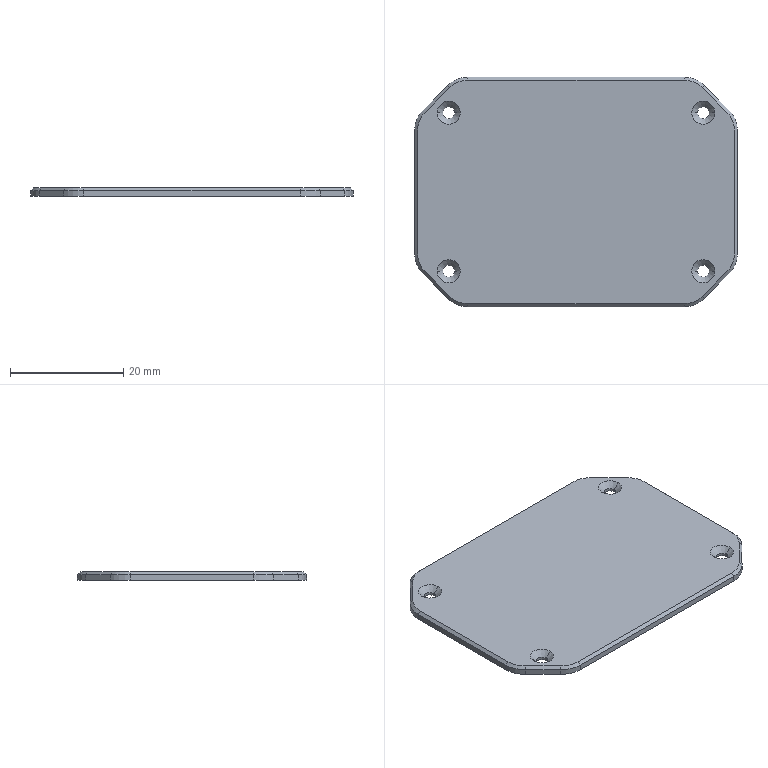NC program | NX | posted with a generic post | part box 57 x 40.5 x 1.5 mm
Lines 1492 to 2967 of 7802:
(PLANAR_PROFILE_COPY_4 , TOOL : D4)
N2916 T01 M6
N2918 G54
N2920 G17 G0 G90 X-245.9 Y31.609 S6500 M3
N2922 G43 Z20. H1
N2924 Z0.1
N2926 G94 G1 Y8.668 Z0.06 F1200.
N2928 X-246.173 Y7.266 Z0.057
N2930 X-246.719 Y5.947 Z0.055
N2932 X-247.518 Y4.763 Z0.052
N2934 X-252.763 Y-0.482 Z0.04
N2936 X-253.947 Y-1.281 Z0.037
N2938 X-255.266 Y-1.827 Z0.035
N2940 X-256.668 Y-2.1 Z0.032
N2942 X-296.332 Z-0.037
N2944 X-297.734 Y-1.827 Z-0.04
N2946 X-299.053 Y-1.281 Z-0.042
N2948 X-300.237 Y-0.482 Z-0.045
N2950 X-305.482 Y4.763 Z-0.058
N2952 X-306.281 Y5.947 Z-0.06
N2954 X-306.827 Y7.266 Z-0.063
N2956 X-307.1 Y8.668 Z-0.065
N2958 Y31.832 Z-0.106
N2960 X-306.827 Y33.234 Z-0.108
N2962 X-306.281 Y34.553 Z-0.11
N2964 X-305.482 Y35.737 Z-0.113
N2966 X-300.237 Y40.982 Z-0.126
N2968 X-299.053 Y41.781 Z-0.128
N2970 X-297.734 Y42.327 Z-0.131
N2972 X-296.332 Y42.6 Z-0.133
N2974 X-256.668 Z-0.203
N2976 X-255.266 Y42.327 Z-0.205
N2978 X-253.947 Y41.781 Z-0.208
N2980 X-252.763 Y40.982 Z-0.21
N2982 X-247.518 Y35.737 Z-0.223
N2984 X-246.719 Y34.553 Z-0.226
N2986 X-246.173 Y33.234 Z-0.228
N2988 X-245.9 Y31.832 Z-0.231
N2990 Y8.668 Z-0.271
N2992 X-246.173 Y7.266 Z-0.273
N2994 X-246.719 Y5.947 Z-0.276
N2996 X-247.518 Y4.763 Z-0.278
N2998 X-252.763 Y-0.482 Z-0.291
N3000 X-253.947 Y-1.281 Z-0.294
N3002 X-255.266 Y-1.827 Z-0.296
N3004 X-256.668 Y-2.1 Z-0.299
N3006 X-257.321 Z-0.3
N3008 X-295.679 F2000.
N3010 G2 X-300.699 Y-0.02 R7.1
N3012 G1 X-305.02 Y4.301
N3014 G2 X-307.1 Y9.321 R7.1
N3016 G1 Y31.179
N3018 G2 X-305.02 Y36.199 R7.1
N3020 G1 X-300.699 Y40.52
N3022 G2 X-295.679 Y42.6 R7.1
N3024 G1 X-257.321
N3026 G2 X-252.301 Y40.52 R7.1
N3028 G1 X-247.98 Y36.199
N3030 G2 X-245.9 Y31.179 R7.1
N3032 G1 Y9.321
N3034 G2 X-247.98 Y4.301 R7.1
N3036 G1 X-252.301 Y-0.02
N3038 G2 X-257.321 Y-2.1 R7.1
N3040 G1 Z-0.2
N3042 G0 Z20.
N3044 X-245.9 Y31.609
N3046 Z-0.2
N3048 G1 Y8.668 Z-0.24 F1200.
N3050 X-246.173 Y7.266 Z-0.243
N3052 X-246.719 Y5.947 Z-0.245
N3054 X-247.518 Y4.763 Z-0.248
N3056 X-252.763 Y-0.482 Z-0.26
N3058 X-253.947 Y-1.281 Z-0.263
N3060 X-255.266 Y-1.827 Z-0.265
N3062 X-256.668 Y-2.1 Z-0.268
N3064 X-296.332 Z-0.337
N3066 X-297.734 Y-1.827 Z-0.34
N3068 X-299.053 Y-1.281 Z-0.342
N3070 X-300.237 Y-0.482 Z-0.345
N3072 X-305.482 Y4.763 Z-0.358
N3074 X-306.281 Y5.947 Z-0.36
N3076 X-306.827 Y7.266 Z-0.363
N3078 X-307.1 Y8.668 Z-0.365
N3080 Y31.832 Z-0.406
N3082 X-306.827 Y33.234 Z-0.408
N3084 X-306.281 Y34.553 Z-0.41
N3086 X-305.482 Y35.737 Z-0.413
N3088 X-300.237 Y40.982 Z-0.426
N3090 X-299.053 Y41.781 Z-0.428
N3092 X-297.734 Y42.327 Z-0.431
N3094 X-296.332 Y42.6 Z-0.433
N3096 X-256.668 Z-0.503
N3098 X-255.266 Y42.327 Z-0.505
N3100 X-253.947 Y41.781 Z-0.508
N3102 X-252.763 Y40.982 Z-0.51
N3104 X-247.518 Y35.737 Z-0.523
N3106 X-246.719 Y34.553 Z-0.526
N3108 X-246.173 Y33.234 Z-0.528
N3110 X-245.9 Y31.832 Z-0.531
N3112 Y8.668 Z-0.571
N3114 X-246.173 Y7.266 Z-0.573
N3116 X-246.719 Y5.947 Z-0.576
N3118 X-247.518 Y4.763 Z-0.578
N3120 X-252.763 Y-0.482 Z-0.591
N3122 X-253.947 Y-1.281 Z-0.594
N3124 X-255.266 Y-1.827 Z-0.596
N3126 X-256.668 Y-2.1 Z-0.599
N3128 X-257.321 Z-0.6
N3130 X-295.679 F2000.
N3132 G2 X-300.699 Y-0.02 R7.1
N3134 G1 X-305.02 Y4.301
N3136 G2 X-307.1 Y9.321 R7.1
N3138 G1 Y31.179
N3140 G2 X-305.02 Y36.199 R7.1
N3142 G1 X-300.699 Y40.52
N3144 G2 X-295.679 Y42.6 R7.1
N3146 G1 X-257.321
N3148 G2 X-252.301 Y40.52 R7.1
N3150 G1 X-247.98 Y36.199
N3152 G2 X-245.9 Y31.179 R7.1
N3154 G1 Y9.321
N3156 G2 X-247.98 Y4.301 R7.1
N3158 G1 X-252.301 Y-0.02
N3160 G2 X-257.321 Y-2.1 R7.1
N3162 G1 Z-0.5
N3164 G0 Z20.
N3166 X-245.9 Y31.609
N3168 Z-0.5
N3170 G1 Y8.668 Z-0.54 F1200.
N3172 X-246.173 Y7.266 Z-0.543
N3174 X-246.719 Y5.947 Z-0.545
N3176 X-247.518 Y4.763 Z-0.548
N3178 X-252.763 Y-0.482 Z-0.56
N3180 X-253.947 Y-1.281 Z-0.563
N3182 X-255.266 Y-1.827 Z-0.565
N3184 X-256.668 Y-2.1 Z-0.568
N3186 X-296.332 Z-0.637
N3188 X-297.734 Y-1.827 Z-0.64
N3190 X-299.053 Y-1.281 Z-0.642
N3192 X-300.237 Y-0.482 Z-0.645
N3194 X-305.482 Y4.763 Z-0.658
N3196 X-306.281 Y5.947 Z-0.66
N3198 X-306.827 Y7.266 Z-0.663
N3200 X-307.1 Y8.668 Z-0.665
N3202 Y31.832 Z-0.706
N3204 X-306.827 Y33.234 Z-0.708
N3206 X-306.281 Y34.553 Z-0.71
N3208 X-305.482 Y35.737 Z-0.713
N3210 X-300.237 Y40.982 Z-0.726
N3212 X-299.053 Y41.781 Z-0.728
N3214 X-297.734 Y42.327 Z-0.731
N3216 X-296.332 Y42.6 Z-0.733
N3218 X-256.668 Z-0.803
N3220 X-255.266 Y42.327 Z-0.805
N3222 X-253.947 Y41.781 Z-0.808
N3224 X-252.763 Y40.982 Z-0.81
N3226 X-247.518 Y35.737 Z-0.823
N3228 X-246.719 Y34.553 Z-0.826
N3230 X-246.173 Y33.234 Z-0.828
N3232 X-245.9 Y31.832 Z-0.831
N3234 Y8.668 Z-0.871
N3236 X-246.173 Y7.266 Z-0.873
N3238 X-246.719 Y5.947 Z-0.876
N3240 X-247.518 Y4.763 Z-0.878
N3242 X-252.763 Y-0.482 Z-0.891
N3244 X-253.947 Y-1.281 Z-0.894
N3246 X-255.266 Y-1.827 Z-0.896
N3248 X-256.668 Y-2.1 Z-0.899
N3250 X-257.321 Z-0.9
N3252 X-295.679 F2000.
N3254 G2 X-300.699 Y-0.02 R7.1
N3256 G1 X-305.02 Y4.301
N3258 G2 X-307.1 Y9.321 R7.1
N3260 G1 Y31.179
N3262 G2 X-305.02 Y36.199 R7.1
N3264 G1 X-300.699 Y40.52
N3266 G2 X-295.679 Y42.6 R7.1
N3268 G1 X-257.321
N3270 G2 X-252.301 Y40.52 R7.1
N3272 G1 X-247.98 Y36.199
N3274 G2 X-245.9 Y31.179 R7.1
N3276 G1 Y9.321
N3278 G2 X-247.98 Y4.301 R7.1
N3280 G1 X-252.301 Y-0.02
N3282 G2 X-257.321 Y-2.1 R7.1
N3284 G1 Z-0.8
N3286 G0 Z20.
N3288 X-245.9 Y31.609
N3290 Z-0.8
N3292 G1 Y8.668 Z-0.84 F1200.
N3294 X-246.173 Y7.266 Z-0.843
N3296 X-246.719 Y5.947 Z-0.845
N3298 X-247.518 Y4.763 Z-0.848
N3300 X-252.763 Y-0.482 Z-0.86
N3302 X-253.947 Y-1.281 Z-0.863
N3304 X-255.266 Y-1.827 Z-0.865
N3306 X-256.668 Y-2.1 Z-0.868
N3308 X-296.332 Z-0.937
N3310 X-297.734 Y-1.827 Z-0.94
N3312 X-299.053 Y-1.281 Z-0.942
N3314 X-300.237 Y-0.482 Z-0.945
N3316 X-305.482 Y4.763 Z-0.958
N3318 X-306.281 Y5.947 Z-0.96
N3320 X-306.827 Y7.266 Z-0.963
N3322 X-307.1 Y8.668 Z-0.965
N3324 Y31.832 Z-1.006
N3326 X-306.827 Y33.234 Z-1.008
N3328 X-306.281 Y34.553 Z-1.01
N3330 X-305.482 Y35.737 Z-1.013
N3332 X-300.237 Y40.982 Z-1.026
N3334 X-299.053 Y41.781 Z-1.028
N3336 X-297.734 Y42.327 Z-1.031
N3338 X-296.332 Y42.6 Z-1.033
N3340 X-256.668 Z-1.103
N3342 X-255.266 Y42.327 Z-1.105
N3344 X-253.947 Y41.781 Z-1.108
N3346 X-252.763 Y40.982 Z-1.11
N3348 X-247.518 Y35.737 Z-1.123
N3350 X-246.719 Y34.553 Z-1.126
N3352 X-246.173 Y33.234 Z-1.128
N3354 X-245.9 Y31.832 Z-1.131
N3356 Y8.668 Z-1.171
N3358 X-246.173 Y7.266 Z-1.173
N3360 X-246.719 Y5.947 Z-1.176
N3362 X-247.518 Y4.763 Z-1.178
N3364 X-252.763 Y-0.482 Z-1.191
N3366 X-253.947 Y-1.281 Z-1.194
N3368 X-255.266 Y-1.827 Z-1.196
N3370 X-256.668 Y-2.1 Z-1.199
N3372 X-257.321 Z-1.2
N3374 X-295.679 F2000.
N3376 G2 X-300.699 Y-0.02 R7.1
N3378 G1 X-305.02 Y4.301
N3380 G2 X-307.1 Y9.321 R7.1
N3382 G1 Y31.179
N3384 G2 X-305.02 Y36.199 R7.1
N3386 G1 X-300.699 Y40.52
N3388 G2 X-295.679 Y42.6 R7.1
N3390 G1 X-257.321
N3392 G2 X-252.301 Y40.52 R7.1
N3394 G1 X-247.98 Y36.199
N3396 G2 X-245.9 Y31.179 R7.1
N3398 G1 Y9.321
N3400 G2 X-247.98 Y4.301 R7.1
N3402 G1 X-252.301 Y-0.02
N3404 G2 X-257.321 Y-2.1 R7.1
N3406 G1 Z-1.1
N3408 G0 Z20.
N3410 X-302.406 Y1.686
N3412 Z-1.1
N3414 G1 X-305.482 Y4.763 Z-1.108 F1200.
N3416 X-306.281 Y5.947 Z-1.11
N3418 X-306.827 Y7.266 Z-1.113
N3420 X-307.1 Y8.668 Z-1.115
N3422 Y31.832 Z-1.156
N3424 X-306.827 Y33.234 Z-1.158
N3426 X-306.281 Y34.553 Z-1.16
N3428 X-305.482 Y35.737 Z-1.163
N3430 X-300.237 Y40.982 Z-1.176
N3432 X-299.053 Y41.781 Z-1.178
N3434 X-297.734 Y42.327 Z-1.181
N3436 X-296.332 Y42.6 Z-1.183
N3438 X-256.668 Z-1.253
N3440 X-255.266 Y42.327 Z-1.255
N3442 X-253.947 Y41.781 Z-1.258
N3444 X-252.763 Y40.982 Z-1.26
N3446 X-247.518 Y35.737 Z-1.273
N3448 X-246.719 Y34.553 Z-1.276
N3450 X-246.173 Y33.234 Z-1.278
N3452 X-245.9 Y31.832 Z-1.281
N3454 Y8.668 Z-1.321
N3456 X-246.173 Y7.266 Z-1.323
N3458 X-246.719 Y5.947 Z-1.326
N3460 X-247.518 Y4.763 Z-1.328
N3462 X-252.763 Y-0.482 Z-1.341
N3464 X-253.947 Y-1.281 Z-1.344
N3466 X-255.266 Y-1.827 Z-1.346
N3468 X-256.668 Y-2.1 Z-1.349
N3470 X-257.321 Z-1.35
N3472 X-295.679 F2000.
N3474 G2 X-300.699 Y-0.02 R7.1
N3476 G1 X-305.02 Y4.301
N3478 G2 X-307.1 Y9.321 R7.1
N3480 G1 Y31.179
N3482 G2 X-305.02 Y36.199 R7.1
N3484 G1 X-300.699 Y40.52
N3486 G2 X-295.679 Y42.6 R7.1
N3488 G1 X-257.321
N3490 G2 X-252.301 Y40.52 R7.1
N3492 G1 X-247.98 Y36.199
N3494 G2 X-245.9 Y31.179 R7.1
N3496 G1 Y9.321
N3498 G2 X-247.98 Y4.301 R7.1
N3500 G1 X-252.301 Y-0.02
N3502 G2 X-257.321 Y-2.1 R7.1
N3504 G1 Z-1.25
N3506 G0 Z20.
(PLANAR_PROFILE_COPY_COPY_4 , TOOL : D4)
N3508 X-257.221
N3510 Z1.65
N3512 G1 Z-1.35 F800.
N3514 X-257.232 Y-2.049
N3516 X-257.27 Y-2.011
N3518 X-257.321 Y-2.
N3520 X-295.679
N3522 G2 X-300.629 Y0.05 R7.
N3524 G1 X-304.95 Y4.371
N3526 G2 X-307. Y9.321 R7.
N3528 G1 Y31.179
N3530 G2 X-304.95 Y36.129 R7.
N3532 G1 X-300.629 Y40.45
N3534 G2 X-295.679 Y42.5 R7.
N3536 G1 X-257.321
N3538 G2 X-252.371 Y40.45 R7.
N3540 G1 X-248.05 Y36.129
N3542 G2 X-246. Y31.179 R7.
N3544 G1 Y9.321
N3546 G2 X-248.05 Y4.371 R7.
N3548 G1 X-252.371 Y0.05
N3550 G2 X-257.321 Y-2. R7.
N3552 G1 X-257.373 Y-2.011
N3554 X-257.41 Y-2.049
N3556 X-257.421 Y-2.1
N3558 Z1.65
N3560 G0 Z20.
N3562 M5
(PLANAR_PROFILE_COPY_COPY_COPY_3 , TOOL : D3倒角)
N3564 T02 M6
N3566 G54
N3568 G17 G0 G90 X-255.321 Y-2.6 S4500 M3
N3570 G43 Z20. H2
N3572 Z2.
N3574 G94 G1 Z-1. F800.
N3576 G3 X-257.321 Y-0.6 R2.
N3578 G1 X-295.679
N3580 G2 X-299.639 Y1.04 R5.6
N3582 G1 X-303.96 Y5.361
N3584 G2 X-305.6 Y9.321 R5.6
N3586 G1 Y31.179
N3588 G2 X-303.96 Y35.139 R5.6
N3590 G1 X-299.639 Y39.46
N3592 G2 X-295.679 Y41.1 R5.6
N3594 G1 X-257.321
N3596 G2 X-253.361 Y39.46 R5.6
N3598 G1 X-249.04 Y35.139
N3600 G2 X-247.4 Y31.179 R5.6
N3602 G1 Y9.321
N3604 G2 X-249.04 Y5.361 R5.6
N3606 G1 X-253.361 Y1.04
N3608 G2 X-257.321 Y-0.6 R5.6
N3610 G3 X-259.321 Y-2.6 R2.
N3612 G1 Z2.
N3614 G0 Z20.
N3616 M5
(PLANAR_PROFILE_COPY_5 , TOOL : D4)
N3618 T01 M6
N3620 G54
N3622 G17 G0 G90 X2.1 Y91.609 S6500 M3
N3624 G43 Z20. H1
N3626 Z0.1
N3628 G94 G1 Y68.668 Z0.06 F1200.
N3630 X1.827 Y67.266 Z0.057
N3632 X1.281 Y65.947 Z0.055
N3634 X0.482 Y64.763 Z0.052
N3636 X-4.763 Y59.518 Z0.04
N3638 X-5.947 Y58.719 Z0.037
N3640 X-7.266 Y58.173 Z0.035
N3642 X-8.668 Y57.9 Z0.032
N3644 X-48.332 Z-0.037
N3646 X-49.734 Y58.173 Z-0.04
N3648 X-51.053 Y58.719 Z-0.042
N3650 X-52.237 Y59.518 Z-0.045
N3652 X-57.482 Y64.763 Z-0.058
N3654 X-58.281 Y65.947 Z-0.06
N3656 X-58.827 Y67.266 Z-0.063
N3658 X-59.1 Y68.668 Z-0.065
N3660 Y91.832 Z-0.106
N3662 X-58.827 Y93.234 Z-0.108
N3664 X-58.281 Y94.553 Z-0.11
N3666 X-57.482 Y95.737 Z-0.113
N3668 X-52.237 Y100.982 Z-0.126
N3670 X-51.053 Y101.781 Z-0.128
N3672 X-49.734 Y102.327 Z-0.131
N3674 X-48.332 Y102.6 Z-0.133
N3676 X-8.668 Z-0.203
N3678 X-7.266 Y102.327 Z-0.205
N3680 X-5.947 Y101.781 Z-0.208
N3682 X-4.763 Y100.982 Z-0.21
N3684 X0.482 Y95.737 Z-0.223
N3686 X1.281 Y94.553 Z-0.226
N3688 X1.827 Y93.234 Z-0.228
N3690 X2.1 Y91.832 Z-0.231
N3692 Y68.668 Z-0.271
N3694 X1.827 Y67.266 Z-0.273
N3696 X1.281 Y65.947 Z-0.276
N3698 X0.482 Y64.763 Z-0.278
N3700 X-4.763 Y59.518 Z-0.291
N3702 X-5.947 Y58.719 Z-0.294
N3704 X-7.266 Y58.173 Z-0.296
N3706 X-8.668 Y57.9 Z-0.299
N3708 X-9.321 Z-0.3
N3710 X-47.679 F2000.
N3712 G2 X-52.699 Y59.98 R7.1
N3714 G1 X-57.02 Y64.301
N3716 G2 X-59.1 Y69.321 R7.1
N3718 G1 Y91.179
N3720 G2 X-57.02 Y96.199 R7.1
N3722 G1 X-52.699 Y100.52
N3724 G2 X-47.679 Y102.6 R7.1
N3726 G1 X-9.321
N3728 G2 X-4.301 Y100.52 R7.1
N3730 G1 X0.02 Y96.199
N3732 G2 X2.1 Y91.179 R7.1
N3734 G1 Y69.321
N3736 G2 X0.02 Y64.301 R7.1
N3738 G1 X-4.301 Y59.98
N3740 G2 X-9.321 Y57.9 R7.1
N3742 G1 Z-0.2
N3744 G0 Z20.
N3746 X2.1 Y91.609
N3748 Z-0.2
N3750 G1 Y68.668 Z-0.24 F1200.
N3752 X1.827 Y67.266 Z-0.243
N3754 X1.281 Y65.947 Z-0.245
N3756 X0.482 Y64.763 Z-0.248
N3758 X-4.763 Y59.518 Z-0.26
N3760 X-5.947 Y58.719 Z-0.263
N3762 X-7.266 Y58.173 Z-0.265
N3764 X-8.668 Y57.9 Z-0.268
N3766 X-48.332 Z-0.337
N3768 X-49.734 Y58.173 Z-0.34
N3770 X-51.053 Y58.719 Z-0.342
N3772 X-52.237 Y59.518 Z-0.345
N3774 X-57.482 Y64.763 Z-0.358
N3776 X-58.281 Y65.947 Z-0.36
N3778 X-58.827 Y67.266 Z-0.363
N3780 X-59.1 Y68.668 Z-0.365
N3782 Y91.832 Z-0.406
N3784 X-58.827 Y93.234 Z-0.408
N3786 X-58.281 Y94.553 Z-0.41
N3788 X-57.482 Y95.737 Z-0.413
N3790 X-52.237 Y100.982 Z-0.426
N3792 X-51.053 Y101.781 Z-0.428
N3794 X-49.734 Y102.327 Z-0.431
N3796 X-48.332 Y102.6 Z-0.433
N3798 X-8.668 Z-0.503
N3800 X-7.266 Y102.327 Z-0.505
N3802 X-5.947 Y101.781 Z-0.508
N3804 X-4.763 Y100.982 Z-0.51
N3806 X0.482 Y95.737 Z-0.523
N3808 X1.281 Y94.553 Z-0.526
N3810 X1.827 Y93.234 Z-0.528
N3812 X2.1 Y91.832 Z-0.531
N3814 Y68.668 Z-0.571
N3816 X1.827 Y67.266 Z-0.573
N3818 X1.281 Y65.947 Z-0.576
N3820 X0.482 Y64.763 Z-0.578
N3822 X-4.763 Y59.518 Z-0.591
N3824 X-5.947 Y58.719 Z-0.594
N3826 X-7.266 Y58.173 Z-0.596
N3828 X-8.668 Y57.9 Z-0.599
N3830 X-9.321 Z-0.6
N3832 X-47.679 F2000.
N3834 G2 X-52.699 Y59.98 R7.1
N3836 G1 X-57.02 Y64.301
N3838 G2 X-59.1 Y69.321 R7.1
N3840 G1 Y91.179
N3842 G2 X-57.02 Y96.199 R7.1
N3844 G1 X-52.699 Y100.52
N3846 G2 X-47.679 Y102.6 R7.1
N3848 G1 X-9.321
N3850 G2 X-4.301 Y100.52 R7.1
N3852 G1 X0.02 Y96.199
N3854 G2 X2.1 Y91.179 R7.1
N3856 G1 Y69.321
N3858 G2 X0.02 Y64.301 R7.1
N3860 G1 X-4.301 Y59.98
N3862 G2 X-9.321 Y57.9 R7.1
N3864 G1 Z-0.5
N3866 G0 Z20.
N3868 X2.1 Y91.609
N3870 Z-0.5
N3872 G1 Y68.668 Z-0.54 F1200.
N3874 X1.827 Y67.266 Z-0.543
N3876 X1.281 Y65.947 Z-0.545
N3878 X0.482 Y64.763 Z-0.548
N3880 X-4.763 Y59.518 Z-0.56
N3882 X-5.947 Y58.719 Z-0.563
N3884 X-7.266 Y58.173 Z-0.565
N3886 X-8.668 Y57.9 Z-0.568
N3888 X-48.332 Z-0.637
N3890 X-49.734 Y58.173 Z-0.64
N3892 X-51.053 Y58.719 Z-0.642
N3894 X-52.237 Y59.518 Z-0.645
N3896 X-57.482 Y64.763 Z-0.658
N3898 X-58.281 Y65.947 Z-0.66
N3900 X-58.827 Y67.266 Z-0.663
N3902 X-59.1 Y68.668 Z-0.665
N3904 Y91.832 Z-0.706
N3906 X-58.827 Y93.234 Z-0.708
N3908 X-58.281 Y94.553 Z-0.71
N3910 X-57.482 Y95.737 Z-0.713
N3912 X-52.237 Y100.982 Z-0.726
N3914 X-51.053 Y101.781 Z-0.728
N3916 X-49.734 Y102.327 Z-0.731
N3918 X-48.332 Y102.6 Z-0.733
N3920 X-8.668 Z-0.803
N3922 X-7.266 Y102.327 Z-0.805
N3924 X-5.947 Y101.781 Z-0.808
N3926 X-4.763 Y100.982 Z-0.81
N3928 X0.482 Y95.737 Z-0.823
N3930 X1.281 Y94.553 Z-0.826
N3932 X1.827 Y93.234 Z-0.828
N3934 X2.1 Y91.832 Z-0.831
N3936 Y68.668 Z-0.871
N3938 X1.827 Y67.266 Z-0.873
N3940 X1.281 Y65.947 Z-0.876
N3942 X0.482 Y64.763 Z-0.878
N3944 X-4.763 Y59.518 Z-0.891
N3946 X-5.947 Y58.719 Z-0.894
N3948 X-7.266 Y58.173 Z-0.896
N3950 X-8.668 Y57.9 Z-0.899
N3952 X-9.321 Z-0.9
N3954 X-47.679 F2000.
N3956 G2 X-52.699 Y59.98 R7.1
N3958 G1 X-57.02 Y64.301
N3960 G2 X-59.1 Y69.321 R7.1
N3962 G1 Y91.179
N3964 G2 X-57.02 Y96.199 R7.1
N3966 G1 X-52.699 Y100.52
N3968 G2 X-47.679 Y102.6 R7.1
N3970 G1 X-9.321
N3972 G2 X-4.301 Y100.52 R7.1
N3974 G1 X0.02 Y96.199
N3976 G2 X2.1 Y91.179 R7.1
N3978 G1 Y69.321
N3980 G2 X0.02 Y64.301 R7.1
N3982 G1 X-4.301 Y59.98
N3984 G2 X-9.321 Y57.9 R7.1
N3986 G1 Z-0.8
N3988 G0 Z20.
N3990 X2.1 Y91.609
N3992 Z-0.8
N3994 G1 Y68.668 Z-0.84 F1200.
N3996 X1.827 Y67.266 Z-0.843
N3998 X1.281 Y65.947 Z-0.845
N4000 X0.482 Y64.763 Z-0.848
N4002 X-4.763 Y59.518 Z-0.86
N4004 X-5.947 Y58.719 Z-0.863
N4006 X-7.266 Y58.173 Z-0.865
N4008 X-8.668 Y57.9 Z-0.868
N4010 X-48.332 Z-0.937
N4012 X-49.734 Y58.173 Z-0.94
N4014 X-51.053 Y58.719 Z-0.942
N4016 X-52.237 Y59.518 Z-0.945
N4018 X-57.482 Y64.763 Z-0.958
N4020 X-58.281 Y65.947 Z-0.96
N4022 X-58.827 Y67.266 Z-0.963
N4024 X-59.1 Y68.668 Z-0.965
N4026 Y91.832 Z-1.006
N4028 X-58.827 Y93.234 Z-1.008
N4030 X-58.281 Y94.553 Z-1.01
N4032 X-57.482 Y95.737 Z-1.013
N4034 X-52.237 Y100.982 Z-1.026
N4036 X-51.053 Y101.781 Z-1.028
N4038 X-49.734 Y102.327 Z-1.031
N4040 X-48.332 Y102.6 Z-1.033
N4042 X-8.668 Z-1.103
N4044 X-7.266 Y102.327 Z-1.105
N4046 X-5.947 Y101.781 Z-1.108
N4048 X-4.763 Y100.982 Z-1.11
N4050 X0.482 Y95.737 Z-1.123
N4052 X1.281 Y94.553 Z-1.126
N4054 X1.827 Y93.234 Z-1.128
N4056 X2.1 Y91.832 Z-1.131
N4058 Y68.668 Z-1.171
N4060 X1.827 Y67.266 Z-1.173
N4062 X1.281 Y65.947 Z-1.176
N4064 X0.482 Y64.763 Z-1.178
N4066 X-4.763 Y59.518 Z-1.191
N4068 X-5.947 Y58.719 Z-1.194
N4070 X-7.266 Y58.173 Z-1.196
N4072 X-8.668 Y57.9 Z-1.199
N4074 X-9.321 Z-1.2
N4076 X-47.679 F2000.
N4078 G2 X-52.699 Y59.98 R7.1
N4080 G1 X-57.02 Y64.301
N4082 G2 X-59.1 Y69.321 R7.1
N4084 G1 Y91.179
N4086 G2 X-57.02 Y96.199 R7.1
N4088 G1 X-52.699 Y100.52
N4090 G2 X-47.679 Y102.6 R7.1
N4092 G1 X-9.321
N4094 G2 X-4.301 Y100.52 R7.1
N4096 G1 X0.02 Y96.199
N4098 G2 X2.1 Y91.179 R7.1
N4100 G1 Y69.321
N4102 G2 X0.02 Y64.301 R7.1
N4104 G1 X-4.301 Y59.98
N4106 G2 X-9.321 Y57.9 R7.1
N4108 G1 Z-1.1
N4110 G0 Z20.
N4112 X2.1 Y91.609
N4114 Z-1.1
N4116 G1 Y68.668 Z-1.14 F1200.
N4118 X1.827 Y67.266 Z-1.143
N4120 X1.281 Y65.947 Z-1.145
N4122 X0.482 Y64.763 Z-1.148
N4124 X-4.763 Y59.518 Z-1.16
N4126 X-5.947 Y58.719 Z-1.163
N4128 X-7.266 Y58.173 Z-1.165
N4130 X-8.668 Y57.9 Z-1.168
N4132 X-48.332 Z-1.237
N4134 X-49.734 Y58.173 Z-1.24
N4136 X-51.053 Y58.719 Z-1.242
N4138 X-52.237 Y59.518 Z-1.245
N4140 X-57.482 Y64.763 Z-1.258
N4142 X-58.281 Y65.947 Z-1.26
N4144 X-58.827 Y67.266 Z-1.263
N4146 X-59.1 Y68.668 Z-1.265
N4148 Y91.832 Z-1.306
N4150 X-58.827 Y93.234 Z-1.308
N4152 X-58.281 Y94.553 Z-1.31
N4154 X-57.482 Y95.737 Z-1.313
N4156 X-52.237 Y100.982 Z-1.326
N4158 X-51.053 Y101.781 Z-1.328
N4160 X-49.734 Y102.327 Z-1.331
N4162 X-48.332 Y102.6 Z-1.333
N4164 X-8.668 Z-1.403
N4166 X-7.266 Y102.327 Z-1.405
N4168 X-5.947 Y101.781 Z-1.408
N4170 X-4.763 Y100.982 Z-1.41
N4172 X0.482 Y95.737 Z-1.423
N4174 X1.281 Y94.553 Z-1.426
N4176 X1.827 Y93.234 Z-1.428
N4178 X2.1 Y91.832 Z-1.431
N4180 Y68.668 Z-1.471
N4182 X1.827 Y67.266 Z-1.473
N4184 X1.281 Y65.947 Z-1.476
N4186 X0.482 Y64.763 Z-1.478
N4188 X-4.763 Y59.518 Z-1.491
N4190 X-5.947 Y58.719 Z-1.494
N4192 X-7.266 Y58.173 Z-1.496
N4194 X-8.668 Y57.9 Z-1.499
N4196 X-9.321 Z-1.5
N4198 X-47.679 F2000.
N4200 G2 X-52.699 Y59.98 R7.1
N4202 G1 X-57.02 Y64.301
N4204 G2 X-59.1 Y69.321 R7.1
N4206 G1 Y91.179
N4208 G2 X-57.02 Y96.199 R7.1
N4210 G1 X-52.699 Y100.52
N4212 G2 X-47.679 Y102.6 R7.1
N4214 G1 X-9.321
N4216 G2 X-4.301 Y100.52 R7.1
N4218 G1 X0.02 Y96.199
N4220 G2 X2.1 Y91.179 R7.1
N4222 G1 Y69.321
N4224 G2 X0.02 Y64.301 R7.1
N4226 G1 X-4.301 Y59.98
N4228 G2 X-9.321 Y57.9 R7.1
N4230 G1 Z-1.4
N4232 G0 Z20.
(PLANAR_PROFILE_COPY_COPY_5 , TOOL : D4)
N4234 X-9.221
N4236 Z1.5
N4238 G1 Z-1.5 F800.
N4240 X-9.232 Y57.952
N4242 X-9.27 Y57.989
N4244 X-9.321 Y58.
N4246 X-47.679
N4248 G2 X-52.629 Y60.05 R7.
N4250 G1 X-56.95 Y64.371
N4252 G2 X-59. Y69.321 R7.
N4254 G1 Y91.179
N4256 G2 X-56.95 Y96.129 R7.
N4258 G1 X-52.629 Y100.45
N4260 G2 X-47.679 Y102.5 R7.
N4262 G1 X-9.321
N4264 G2 X-4.371 Y100.45 R7.
N4266 G1 X-0.05 Y96.129
N4268 G2 X2. Y91.179 R7.
N4270 G1 Y69.321
N4272 G2 X-0.05 Y64.371 R7.
N4274 G1 X-4.371 Y60.05
N4276 G2 X-9.321 Y58. R7.
N4278 G1 X-9.373 Y57.989
N4280 X-9.41 Y57.952
N4282 X-9.421 Y57.9
N4284 Z1.5
N4286 G0 Z20.
N4288 M5
(PLANAR_PROFILE_COPY_COPY_COPY_4 , TOOL : D3倒角)
N4290 T02 M6
N4292 G54
N4294 G17 G0 G90 X-7.321 Y57.4 S4500 M3
N4296 G43 Z20. H2
N4298 Z2.
N4300 G94 G1 Z-1. F800.
N4302 G3 X-9.321 Y59.4 R2.
N4304 G1 X-47.679
N4306 G2 X-51.639 Y61.04 R5.6
N4308 G1 X-55.96 Y65.361
N4310 G2 X-57.6 Y69.321 R5.6
N4312 G1 Y91.179
N4314 G2 X-55.96 Y95.139 R5.6
N4316 G1 X-51.639 Y99.46
N4318 G2 X-47.679 Y101.1 R5.6
N4320 G1 X-9.321
N4322 G2 X-5.361 Y99.46 R5.6
N4324 G1 X-1.04 Y95.139
N4326 G2 X0.6 Y91.179 R5.6
N4328 G1 Y69.321
N4330 G2 X-1.04 Y65.361 R5.6
N4332 G1 X-5.361 Y61.04
N4334 G2 X-9.321 Y59.4 R5.6
N4336 G3 X-11.321 Y57.4 R2.
N4338 G1 Z2.
N4340 G0 Z20.
N4342 M5
(PLANAR_PROFILE_COPY_1_COPY , TOOL : D4)
N4344 T01 M6
N4346 G54
N4348 G17 G0 G90 X-59.9 Y91.609 S6500 M3
N4350 G43 Z20. H1
N4352 Z0.1
N4354 G94 G1 Y68.668 Z0.06 F1200.
N4356 X-60.173 Y67.266 Z0.057
N4358 X-60.719 Y65.947 Z0.055
N4360 X-61.518 Y64.763 Z0.052
N4362 X-66.763 Y59.518 Z0.04
N4364 X-67.947 Y58.719 Z0.037
N4366 X-69.266 Y58.173 Z0.035
N4368 X-70.668 Y57.9 Z0.032
N4370 X-110.332 Z-0.037
N4372 X-111.734 Y58.173 Z-0.04
N4374 X-113.053 Y58.719 Z-0.042
N4376 X-114.237 Y59.518 Z-0.045
N4378 X-119.482 Y64.763 Z-0.058
N4380 X-120.281 Y65.947 Z-0.06
N4382 X-120.827 Y67.266 Z-0.063
N4384 X-121.1 Y68.668 Z-0.065
N4386 Y91.832 Z-0.106
N4388 X-120.827 Y93.234 Z-0.108
N4390 X-120.281 Y94.553 Z-0.11
N4392 X-119.482 Y95.737 Z-0.113
N4394 X-114.237 Y100.982 Z-0.126
N4396 X-113.053 Y101.781 Z-0.128
N4398 X-111.734 Y102.327 Z-0.131
N4400 X-110.332 Y102.6 Z-0.133
N4402 X-70.668 Z-0.203
N4404 X-69.266 Y102.327 Z-0.205
N4406 X-67.947 Y101.781 Z-0.208
N4408 X-66.763 Y100.982 Z-0.21
N4410 X-61.518 Y95.737 Z-0.223
N4412 X-60.719 Y94.553 Z-0.226
N4414 X-60.173 Y93.234 Z-0.228
N4416 X-59.9 Y91.832 Z-0.231
N4418 Y68.668 Z-0.271
N4420 X-60.173 Y67.266 Z-0.273
N4422 X-60.719 Y65.947 Z-0.276
N4424 X-61.518 Y64.763 Z-0.278
N4426 X-66.763 Y59.518 Z-0.291
N4428 X-67.947 Y58.719 Z-0.294
N4430 X-69.266 Y58.173 Z-0.296
N4432 X-70.668 Y57.9 Z-0.299
N4434 X-71.321 Z-0.3
N4436 X-109.679 F2000.
N4438 G2 X-114.699 Y59.98 R7.1
N4440 G1 X-119.02 Y64.301
N4442 G2 X-121.1 Y69.321 R7.1
N4444 G1 Y91.179
N4446 G2 X-119.02 Y96.199 R7.1
N4448 G1 X-114.699 Y100.52
N4450 G2 X-109.679 Y102.6 R7.1
N4452 G1 X-71.321
N4454 G2 X-66.301 Y100.52 R7.1
N4456 G1 X-61.98 Y96.199
N4458 G2 X-59.9 Y91.179 R7.1
N4460 G1 Y69.321
N4462 G2 X-61.98 Y64.301 R7.1
N4464 G1 X-66.301 Y59.98
N4466 G2 X-71.321 Y57.9 R7.1
N4468 G1 Z-0.2
N4470 G0 Z20.
N4472 X-59.9 Y91.609
N4474 Z-0.2
N4476 G1 Y68.668 Z-0.24 F1200.
N4478 X-60.173 Y67.266 Z-0.243
N4480 X-60.719 Y65.947 Z-0.245
N4482 X-61.518 Y64.763 Z-0.248
N4484 X-66.763 Y59.518 Z-0.26
N4486 X-67.947 Y58.719 Z-0.263
N4488 X-69.266 Y58.173 Z-0.265
N4490 X-70.668 Y57.9 Z-0.268
N4492 X-110.332 Z-0.337
N4494 X-111.734 Y58.173 Z-0.34
N4496 X-113.053 Y58.719 Z-0.342
N4498 X-114.237 Y59.518 Z-0.345
N4500 X-119.482 Y64.763 Z-0.358
N4502 X-120.281 Y65.947 Z-0.36
N4504 X-120.827 Y67.266 Z-0.363
N4506 X-121.1 Y68.668 Z-0.365
N4508 Y91.832 Z-0.406
N4510 X-120.827 Y93.234 Z-0.408
N4512 X-120.281 Y94.553 Z-0.41
N4514 X-119.482 Y95.737 Z-0.413
N4516 X-114.237 Y100.982 Z-0.426
N4518 X-113.053 Y101.781 Z-0.428
N4520 X-111.734 Y102.327 Z-0.431
N4522 X-110.332 Y102.6 Z-0.433
N4524 X-70.668 Z-0.503
N4526 X-69.266 Y102.327 Z-0.505
N4528 X-67.947 Y101.781 Z-0.508
N4530 X-66.763 Y100.982 Z-0.51
N4532 X-61.518 Y95.737 Z-0.523
N4534 X-60.719 Y94.553 Z-0.526
N4536 X-60.173 Y93.234 Z-0.528
N4538 X-59.9 Y91.832 Z-0.531
N4540 Y68.668 Z-0.571
N4542 X-60.173 Y67.266 Z-0.573
N4544 X-60.719 Y65.947 Z-0.576
N4546 X-61.518 Y64.763 Z-0.578
N4548 X-66.763 Y59.518 Z-0.591
N4550 X-67.947 Y58.719 Z-0.594
N4552 X-69.266 Y58.173 Z-0.596
N4554 X-70.668 Y57.9 Z-0.599
N4556 X-71.321 Z-0.6
N4558 X-109.679 F2000.
N4560 G2 X-114.699 Y59.98 R7.1
N4562 G1 X-119.02 Y64.301
N4564 G2 X-121.1 Y69.321 R7.1
N4566 G1 Y91.179
N4568 G2 X-119.02 Y96.199 R7.1
N4570 G1 X-114.699 Y100.52
N4572 G2 X-109.679 Y102.6 R7.1
N4574 G1 X-71.321
N4576 G2 X-66.301 Y100.52 R7.1
N4578 G1 X-61.98 Y96.199
N4580 G2 X-59.9 Y91.179 R7.1
N4582 G1 Y69.321
N4584 G2 X-61.98 Y64.301 R7.1
N4586 G1 X-66.301 Y59.98
N4588 G2 X-71.321 Y57.9 R7.1
N4590 G1 Z-0.5
N4592 G0 Z20.
N4594 X-59.9 Y91.609
N4596 Z-0.5
N4598 G1 Y68.668 Z-0.54 F1200.
N4600 X-60.173 Y67.266 Z-0.543
N4602 X-60.719 Y65.947 Z-0.545
N4604 X-61.518 Y64.763 Z-0.548
N4606 X-66.763 Y59.518 Z-0.56
N4608 X-67.947 Y58.719 Z-0.563
N4610 X-69.266 Y58.173 Z-0.565
N4612 X-70.668 Y57.9 Z-0.568
N4614 X-110.332 Z-0.637
N4616 X-111.734 Y58.173 Z-0.64
N4618 X-113.053 Y58.719 Z-0.642
N4620 X-114.237 Y59.518 Z-0.645
N4622 X-119.482 Y64.763 Z-0.658
N4624 X-120.281 Y65.947 Z-0.66
N4626 X-120.827 Y67.266 Z-0.663
N4628 X-121.1 Y68.668 Z-0.665
N4630 Y91.832 Z-0.706
N4632 X-120.827 Y93.234 Z-0.708
N4634 X-120.281 Y94.553 Z-0.71
N4636 X-119.482 Y95.737 Z-0.713
N4638 X-114.237 Y100.982 Z-0.726
N4640 X-113.053 Y101.781 Z-0.728
N4642 X-111.734 Y102.327 Z-0.731
N4644 X-110.332 Y102.6 Z-0.733
N4646 X-70.668 Z-0.803
N4648 X-69.266 Y102.327 Z-0.805
N4650 X-67.947 Y101.781 Z-0.808
N4652 X-66.763 Y100.982 Z-0.81
N4654 X-61.518 Y95.737 Z-0.823
N4656 X-60.719 Y94.553 Z-0.826
N4658 X-60.173 Y93.234 Z-0.828
N4660 X-59.9 Y91.832 Z-0.831
N4662 Y68.668 Z-0.871
N4664 X-60.173 Y67.266 Z-0.873
N4666 X-60.719 Y65.947 Z-0.876
N4668 X-61.518 Y64.763 Z-0.878
N4670 X-66.763 Y59.518 Z-0.891
N4672 X-67.947 Y58.719 Z-0.894
N4674 X-69.266 Y58.173 Z-0.896
N4676 X-70.668 Y57.9 Z-0.899
N4678 X-71.321 Z-0.9
N4680 X-109.679 F2000.
N4682 G2 X-114.699 Y59.98 R7.1
N4684 G1 X-119.02 Y64.301
N4686 G2 X-121.1 Y69.321 R7.1
N4688 G1 Y91.179
N4690 G2 X-119.02 Y96.199 R7.1
N4692 G1 X-114.699 Y100.52
N4694 G2 X-109.679 Y102.6 R7.1
N4696 G1 X-71.321
N4698 G2 X-66.301 Y100.52 R7.1
N4700 G1 X-61.98 Y96.199
N4702 G2 X-59.9 Y91.179 R7.1
N4704 G1 Y69.321
N4706 G2 X-61.98 Y64.301 R7.1
N4708 G1 X-66.301 Y59.98
N4710 G2 X-71.321 Y57.9 R7.1
N4712 G1 Z-0.8
N4714 G0 Z20.
N4716 X-59.9 Y91.609
N4718 Z-0.8
N4720 G1 Y68.668 Z-0.84 F1200.
N4722 X-60.173 Y67.266 Z-0.843
N4724 X-60.719 Y65.947 Z-0.845
N4726 X-61.518 Y64.763 Z-0.848
N4728 X-66.763 Y59.518 Z-0.86
N4730 X-67.947 Y58.719 Z-0.863
N4732 X-69.266 Y58.173 Z-0.865
N4734 X-70.668 Y57.9 Z-0.868
N4736 X-110.332 Z-0.937
N4738 X-111.734 Y58.173 Z-0.94
N4740 X-113.053 Y58.719 Z-0.942
N4742 X-114.237 Y59.518 Z-0.945
N4744 X-119.482 Y64.763 Z-0.958
N4746 X-120.281 Y65.947 Z-0.96
N4748 X-120.827 Y67.266 Z-0.963
N4750 X-121.1 Y68.668 Z-0.965
N4752 Y91.832 Z-1.006
N4754 X-120.827 Y93.234 Z-1.008
N4756 X-120.281 Y94.553 Z-1.01
N4758 X-119.482 Y95.737 Z-1.013
N4760 X-114.237 Y100.982 Z-1.026
N4762 X-113.053 Y101.781 Z-1.028
N4764 X-111.734 Y102.327 Z-1.031
N4766 X-110.332 Y102.6 Z-1.033
N4768 X-70.668 Z-1.103
N4770 X-69.266 Y102.327 Z-1.105
N4772 X-67.947 Y101.781 Z-1.108
N4774 X-66.763 Y100.982 Z-1.11
N4776 X-61.518 Y95.737 Z-1.123
N4778 X-60.719 Y94.553 Z-1.126
N4780 X-60.173 Y93.234 Z-1.128
N4782 X-59.9 Y91.832 Z-1.131
N4784 Y68.668 Z-1.171
N4786 X-60.173 Y67.266 Z-1.173
N4788 X-60.719 Y65.947 Z-1.176
N4790 X-61.518 Y64.763 Z-1.178
N4792 X-66.763 Y59.518 Z-1.191
N4794 X-67.947 Y58.719 Z-1.194
N4796 X-69.266 Y58.173 Z-1.196
N4798 X-70.668 Y57.9 Z-1.199
N4800 X-71.321 Z-1.2
N4802 X-109.679 F2000.
N4804 G2 X-114.699 Y59.98 R7.1
N4806 G1 X-119.02 Y64.301
N4808 G2 X-121.1 Y69.321 R7.1
N4810 G1 Y91.179
N4812 G2 X-119.02 Y96.199 R7.1
N4814 G1 X-114.699 Y100.52
N4816 G2 X-109.679 Y102.6 R7.1
N4818 G1 X-71.321
N4820 G2 X-66.301 Y100.52 R7.1
N4822 G1 X-61.98 Y96.199
N4824 G2 X-59.9 Y91.179 R7.1
N4826 G1 Y69.321
N4828 G2 X-61.98 Y64.301 R7.1
N4830 G1 X-66.301 Y59.98
N4832 G2 X-71.321 Y57.9 R7.1
N4834 G1 Z-1.1
N4836 G0 Z20.
N4838 X-59.9 Y91.609
N4840 Z-1.1
N4842 G1 Y68.668 Z-1.14 F1200.
N4844 X-60.173 Y67.266 Z-1.143
N4846 X-60.719 Y65.947 Z-1.145
N4848 X-61.518 Y64.763 Z-1.148
N4850 X-66.763 Y59.518 Z-1.16
N4852 X-67.947 Y58.719 Z-1.163
N4854 X-69.266 Y58.173 Z-1.165
N4856 X-70.668 Y57.9 Z-1.168
N4858 X-110.332 Z-1.237
N4860 X-111.734 Y58.173 Z-1.24
N4862 X-113.053 Y58.719 Z-1.242
N4864 X-114.237 Y59.518 Z-1.245
N4866 X-119.482 Y64.763 Z-1.258
N4868 X-120.281 Y65.947 Z-1.26
N4870 X-120.827 Y67.266 Z-1.263
N4872 X-121.1 Y68.668 Z-1.265
N4874 Y91.832 Z-1.306
N4876 X-120.827 Y93.234 Z-1.308
N4878 X-120.281 Y94.553 Z-1.31
N4880 X-119.482 Y95.737 Z-1.313
N4882 X-114.237 Y100.982 Z-1.326
N4884 X-113.053 Y101.781 Z-1.328
N4886 X-111.734 Y102.327 Z-1.331
N4888 X-110.332 Y102.6 Z-1.333
N4890 X-70.668 Z-1.403
N4892 X-69.266 Y102.327 Z-1.405
N4894 X-67.947 Y101.781 Z-1.408
N4896 X-66.763 Y100.982 Z-1.41
N4898 X-61.518 Y95.737 Z-1.423
N4900 X-60.719 Y94.553 Z-1.426
N4902 X-60.173 Y93.234 Z-1.428
N4904 X-59.9 Y91.832 Z-1.431
N4906 Y68.668 Z-1.471
N4908 X-60.173 Y67.266 Z-1.473
N4910 X-60.719 Y65.947 Z-1.476
N4912 X-61.518 Y64.763 Z-1.478
N4914 X-66.763 Y59.518 Z-1.491
N4916 X-67.947 Y58.719 Z-1.494
N4918 X-69.266 Y58.173 Z-1.496
N4920 X-70.668 Y57.9 Z-1.499
N4922 X-71.321 Z-1.5
N4924 X-109.679 F2000.
N4926 G2 X-114.699 Y59.98 R7.1
N4928 G1 X-119.02 Y64.301
N4930 G2 X-121.1 Y69.321 R7.1
N4932 G1 Y91.179
N4934 G2 X-119.02 Y96.199 R7.1
N4936 G1 X-114.699 Y100.52
N4938 G2 X-109.679 Y102.6 R7.1
N4940 G1 X-71.321
N4942 G2 X-66.301 Y100.52 R7.1
N4944 G1 X-61.98 Y96.199
N4946 G2 X-59.9 Y91.179 R7.1
N4948 G1 Y69.321
N4950 G2 X-61.98 Y64.301 R7.1
N4952 G1 X-66.301 Y59.98
N4954 G2 X-71.321 Y57.9 R7.1
N4956 G1 Z-1.4
N4958 G0 Z20.
(PLANAR_PROFILE_COPY_COPY_1_COPY , TOOL : D4)
N4960 X-71.221
N4962 Z1.5
N4964 G1 Z-1.5 F800.
N4966 X-71.232 Y57.952
N4968 X-71.27 Y57.989
N4970 X-71.321 Y58.
N4972 X-109.679
N4974 G2 X-114.629 Y60.05 R7.
N4976 G1 X-118.95 Y64.371
N4978 G2 X-121. Y69.321 R7.
N4980 G1 Y91.179
N4982 G2 X-118.95 Y96.129 R7.
N4984 G1 X-114.629 Y100.45
N4986 G2 X-109.679 Y102.5 R7.
N4988 G1 X-71.321
N4990 G2 X-66.371 Y100.45 R7.
N4992 G1 X-62.05 Y96.129
N4994 G2 X-60. Y91.179 R7.
N4996 G1 Y69.321
N4998 G2 X-62.05 Y64.371 R7.
N5000 G1 X-66.371 Y60.05
N5002 G2 X-71.321 Y58. R7.
N5004 G1 X-71.373 Y57.989
N5006 X-71.41 Y57.952
N5008 X-71.421 Y57.9
N5010 Z1.5
N5012 G0 Z20.
N5014 M5
(PLANAR_PROFILE_COPY_COPY_COPY_COPY , TOOL : D3倒角)
N5016 T02 M6
N5018 G54
N5020 G17 G0 G90 X-69.321 Y57.4 S4500 M3
N5022 G43 Z20. H2
N5024 Z2.
N5026 G94 G1 Z-1. F800.
N5028 G3 X-71.321 Y59.4 R2.
N5030 G1 X-109.679
N5032 G2 X-113.639 Y61.04 R5.6
N5034 G1 X-117.96 Y65.361
N5036 G2 X-119.6 Y69.321 R5.6
N5038 G1 Y91.179
N5040 G2 X-117.96 Y95.139 R5.6
N5042 G1 X-113.639 Y99.46
N5044 G2 X-109.679 Y101.1 R5.6
N5046 G1 X-71.321
N5048 G2 X-67.361 Y99.46 R5.6
N5050 G1 X-63.04 Y95.139
N5052 G2 X-61.4 Y91.179 R5.6
N5054 G1 Y69.321
N5056 G2 X-63.04 Y65.361 R5.6
N5058 G1 X-67.361 Y61.04
N5060 G2 X-71.321 Y59.4 R5.6
N5062 G3 X-73.321 Y57.4 R2.
N5064 G1 Z2.
N5066 G0 Z20.
N5068 M5
(PLANAR_PROFILE_COPY_2_COPY , TOOL : D4)
N5070 T01 M6
N5072 G54
N5074 G17 G0 G90 X-121.9 Y91.609 S6500 M3
N5076 G43 Z20. H1
N5078 Z0.1
N5080 G94 G1 Y68.668 Z0.06 F1200.
N5082 X-122.173 Y67.266 Z0.057
N5084 X-122.719 Y65.947 Z0.055
N5086 X-123.518 Y64.763 Z0.052
N5088 X-128.763 Y59.518 Z0.04
N5090 X-129.947 Y58.719 Z0.037
N5092 X-131.266 Y58.173 Z0.035
N5094 X-132.668 Y57.9 Z0.032
N5096 X-172.332 Z-0.037
N5098 X-173.734 Y58.173 Z-0.04
N5100 X-175.053 Y58.719 Z-0.042
N5102 X-176.237 Y59.518 Z-0.045
N5104 X-181.482 Y64.763 Z-0.058
N5106 X-182.281 Y65.947 Z-0.06
N5108 X-182.827 Y67.266 Z-0.063
N5110 X-183.1 Y68.668 Z-0.065
N5112 Y91.832 Z-0.106
N5114 X-182.827 Y93.234 Z-0.108
N5116 X-182.281 Y94.553 Z-0.11
N5118 X-181.482 Y95.737 Z-0.113
N5120 X-176.237 Y100.982 Z-0.126
N5122 X-175.053 Y101.781 Z-0.128
N5124 X-173.734 Y102.327 Z-0.131
N5126 X-172.332 Y102.6 Z-0.133
N5128 X-132.668 Z-0.203
N5130 X-131.266 Y102.327 Z-0.205
N5132 X-129.947 Y101.781 Z-0.208
N5134 X-128.763 Y100.982 Z-0.21
N5136 X-123.518 Y95.737 Z-0.223
N5138 X-122.719 Y94.553 Z-0.226
N5140 X-122.173 Y93.234 Z-0.228
N5142 X-121.9 Y91.832 Z-0.231
N5144 Y68.668 Z-0.271
N5146 X-122.173 Y67.266 Z-0.273
N5148 X-122.719 Y65.947 Z-0.276
N5150 X-123.518 Y64.763 Z-0.278
N5152 X-128.763 Y59.518 Z-0.291
N5154 X-129.947 Y58.719 Z-0.294
N5156 X-131.266 Y58.173 Z-0.296
N5158 X-132.668 Y57.9 Z-0.299
N5160 X-133.321 Z-0.3
N5162 X-171.679 F2000.
N5164 G2 X-176.699 Y59.98 R7.1
N5166 G1 X-181.02 Y64.301
N5168 G2 X-183.1 Y69.321 R7.1
N5170 G1 Y91.179
N5172 G2 X-181.02 Y96.199 R7.1
N5174 G1 X-176.699 Y100.52
N5176 G2 X-171.679 Y102.6 R7.1
N5178 G1 X-133.321
N5180 G2 X-128.301 Y100.52 R7.1
N5182 G1 X-123.98 Y96.199
N5184 G2 X-121.9 Y91.179 R7.1
N5186 G1 Y69.321
N5188 G2 X-123.98 Y64.301 R7.1
N5190 G1 X-128.301 Y59.98
N5192 G2 X-133.321 Y57.9 R7.1
N5194 G1 Z-0.2
N5196 G0 Z20.
N5198 X-121.9 Y91.609
N5200 Z-0.2
N5202 G1 Y68.668 Z-0.24 F1200.
N5204 X-122.173 Y67.266 Z-0.243
N5206 X-122.719 Y65.947 Z-0.245
N5208 X-123.518 Y64.763 Z-0.248
N5210 X-128.763 Y59.518 Z-0.26
N5212 X-129.947 Y58.719 Z-0.263
N5214 X-131.266 Y58.173 Z-0.265
N5216 X-132.668 Y57.9 Z-0.268
N5218 X-172.332 Z-0.337
N5220 X-173.734 Y58.173 Z-0.34
N5222 X-175.053 Y58.719 Z-0.342
N5224 X-176.237 Y59.518 Z-0.345
N5226 X-181.482 Y64.763 Z-0.358
N5228 X-182.281 Y65.947 Z-0.36
N5230 X-182.827 Y67.266 Z-0.363
N5232 X-183.1 Y68.668 Z-0.365
N5234 Y91.832 Z-0.406
N5236 X-182.827 Y93.234 Z-0.408
N5238 X-182.281 Y94.553 Z-0.41
N5240 X-181.482 Y95.737 Z-0.413
N5242 X-176.237 Y100.982 Z-0.426
N5244 X-175.053 Y101.781 Z-0.428
N5246 X-173.734 Y102.327 Z-0.431
N5248 X-172.332 Y102.6 Z-0.433
N5250 X-132.668 Z-0.503
N5252 X-131.266 Y102.327 Z-0.505
N5254 X-129.947 Y101.781 Z-0.508
N5256 X-128.763 Y100.982 Z-0.51
N5258 X-123.518 Y95.737 Z-0.523
N5260 X-122.719 Y94.553 Z-0.526
N5262 X-122.173 Y93.234 Z-0.528
N5264 X-121.9 Y91.832 Z-0.531
N5266 Y68.668 Z-0.571
N5268 X-122.173 Y67.266 Z-0.573
N5270 X-122.719 Y65.947 Z-0.576
N5272 X-123.518 Y64.763 Z-0.578
N5274 X-128.763 Y59.518 Z-0.591
N5276 X-129.947 Y58.719 Z-0.594
N5278 X-131.266 Y58.173 Z-0.596
N5280 X-132.668 Y57.9 Z-0.599
N5282 X-133.321 Z-0.6
N5284 X-171.679 F2000.
N5286 G2 X-176.699 Y59.98 R7.1
N5288 G1 X-181.02 Y64.301
N5290 G2 X-183.1 Y69.321 R7.1
N5292 G1 Y91.179
N5294 G2 X-181.02 Y96.199 R7.1
N5296 G1 X-176.699 Y100.52
N5298 G2 X-171.679 Y102.6 R7.1
N5300 G1 X-133.321
N5302 G2 X-128.301 Y100.52 R7.1
N5304 G1 X-123.98 Y96.199
N5306 G2 X-121.9 Y91.179 R7.1
N5308 G1 Y69.321
N5310 G2 X-123.98 Y64.301 R7.1
N5312 G1 X-128.301 Y59.98
N5314 G2 X-133.321 Y57.9 R7.1
N5316 G1 Z-0.5
N5318 G0 Z20.
N5320 X-121.9 Y91.609
N5322 Z-0.5
N5324 G1 Y68.668 Z-0.54 F1200.
N5326 X-122.173 Y67.266 Z-0.543
N5328 X-122.719 Y65.947 Z-0.545
N5330 X-123.518 Y64.763 Z-0.548
N5332 X-128.763 Y59.518 Z-0.56
N5334 X-129.947 Y58.719 Z-0.563
N5336 X-131.266 Y58.173 Z-0.565
N5338 X-132.668 Y57.9 Z-0.568
N5340 X-172.332 Z-0.637
N5342 X-173.734 Y58.173 Z-0.64
N5344 X-175.053 Y58.719 Z-0.642
N5346 X-176.237 Y59.518 Z-0.645
N5348 X-181.482 Y64.763 Z-0.658
N5350 X-182.281 Y65.947 Z-0.66
N5352 X-182.827 Y67.266 Z-0.663
N5354 X-183.1 Y68.668 Z-0.665
N5356 Y91.832 Z-0.706
N5358 X-182.827 Y93.234 Z-0.708
N5360 X-182.281 Y94.553 Z-0.71
N5362 X-181.482 Y95.737 Z-0.713
N5364 X-176.237 Y100.982 Z-0.726
N5366 X-175.053 Y101.781 Z-0.728
N5368 X-173.734 Y102.327 Z-0.731
N5370 X-172.332 Y102.6 Z-0.733
N5372 X-132.668 Z-0.803
N5374 X-131.266 Y102.327 Z-0.805
N5376 X-129.947 Y101.781 Z-0.808
N5378 X-128.763 Y100.982 Z-0.81
N5380 X-123.518 Y95.737 Z-0.823
N5382 X-122.719 Y94.553 Z-0.826
N5384 X-122.173 Y93.234 Z-0.828
N5386 X-121.9 Y91.832 Z-0.831
N5388 Y68.668 Z-0.871
N5390 X-122.173 Y67.266 Z-0.873
N5392 X-122.719 Y65.947 Z-0.876
N5394 X-123.518 Y64.763 Z-0.878
N5396 X-128.763 Y59.518 Z-0.891
N5398 X-129.947 Y58.719 Z-0.894
N5400 X-131.266 Y58.173 Z-0.896
N5402 X-132.668 Y57.9 Z-0.899
N5404 X-133.321 Z-0.9
N5406 X-171.679 F2000.
N5408 G2 X-176.699 Y59.98 R7.1
N5410 G1 X-181.02 Y64.301
N5412 G2 X-183.1 Y69.321 R7.1
N5414 G1 Y91.179
N5416 G2 X-181.02 Y96.199 R7.1
N5418 G1 X-176.699 Y100.52
N5420 G2 X-171.679 Y102.6 R7.1
N5422 G1 X-133.321
N5424 G2 X-128.301 Y100.52 R7.1
N5426 G1 X-123.98 Y96.199
N5428 G2 X-121.9 Y91.179 R7.1
N5430 G1 Y69.321
N5432 G2 X-123.98 Y64.301 R7.1
N5434 G1 X-128.301 Y59.98
N5436 G2 X-133.321 Y57.9 R7.1
N5438 G1 Z-0.8
N5440 G0 Z20.
N5442 X-121.9 Y91.609
N5444 Z-0.8
N5446 G1 Y68.668 Z-0.84 F1200.
N5448 X-122.173 Y67.266 Z-0.843
N5450 X-122.719 Y65.947 Z-0.845
N5452 X-123.518 Y64.763 Z-0.848
N5454 X-128.763 Y59.518 Z-0.86
N5456 X-129.947 Y58.719 Z-0.863
N5458 X-131.266 Y58.173 Z-0.865
N5460 X-132.668 Y57.9 Z-0.868
N5462 X-172.332 Z-0.937
N5464 X-173.734 Y58.173 Z-0.94
N5466 X-175.053 Y58.719 Z-0.942
N5468 X-176.237 Y59.518 Z-0.945
N5470 X-181.482 Y64.763 Z-0.958
N5472 X-182.281 Y65.947 Z-0.96
N5474 X-182.827 Y67.266 Z-0.963
N5476 X-183.1 Y68.668 Z-0.965
N5478 Y91.832 Z-1.006
N5480 X-182.827 Y93.234 Z-1.008
N5482 X-182.281 Y94.553 Z-1.01
N5484 X-181.482 Y95.737 Z-1.013
N5486 X-176.237 Y100.982 Z-1.026
N5488 X-175.053 Y101.781 Z-1.028
N5490 X-173.734 Y102.327 Z-1.031
N5492 X-172.332 Y102.6 Z-1.033
N5494 X-132.668 Z-1.103
N5496 X-131.266 Y102.327 Z-1.105
N5498 X-129.947 Y101.781 Z-1.108
N5500 X-128.763 Y100.982 Z-1.11
N5502 X-123.518 Y95.737 Z-1.123
N5504 X-122.719 Y94.553 Z-1.126
N5506 X-122.173 Y93.234 Z-1.128
N5508 X-121.9 Y91.832 Z-1.131
N5510 Y68.668 Z-1.171
N5512 X-122.173 Y67.266 Z-1.173
N5514 X-122.719 Y65.947 Z-1.176
N5516 X-123.518 Y64.763 Z-1.178
N5518 X-128.763 Y59.518 Z-1.191
N5520 X-129.947 Y58.719 Z-1.194
N5522 X-131.266 Y58.173 Z-1.196
N5524 X-132.668 Y57.9 Z-1.199
N5526 X-133.321 Z-1.2
N5528 X-171.679 F2000.
N5530 G2 X-176.699 Y59.98 R7.1
N5532 G1 X-181.02 Y64.301
N5534 G2 X-183.1 Y69.321 R7.1
N5536 G1 Y91.179
N5538 G2 X-181.02 Y96.199 R7.1
N5540 G1 X-176.699 Y100.52
N5542 G2 X-171.679 Y102.6 R7.1
N5544 G1 X-133.321
N5546 G2 X-128.301 Y100.52 R7.1
N5548 G1 X-123.98 Y96.199
N5550 G2 X-121.9 Y91.179 R7.1
N5552 G1 Y69.321
N5554 G2 X-123.98 Y64.301 R7.1
N5556 G1 X-128.301 Y59.98
N5558 G2 X-133.321 Y57.9 R7.1
N5560 G1 Z-1.1
N5562 G0 Z20.
N5564 X-121.9 Y91.609
N5566 Z-1.1
N5568 G1 Y68.668 Z-1.14 F1200.
N5570 X-122.173 Y67.266 Z-1.143
N5572 X-122.719 Y65.947 Z-1.145
N5574 X-123.518 Y64.763 Z-1.148
N5576 X-128.763 Y59.518 Z-1.16
N5578 X-129.947 Y58.719 Z-1.163
N5580 X-131.266 Y58.173 Z-1.165
N5582 X-132.668 Y57.9 Z-1.168
N5584 X-172.332 Z-1.237
N5586 X-173.734 Y58.173 Z-1.24
N5588 X-175.053 Y58.719 Z-1.242
N5590 X-176.237 Y59.518 Z-1.245
N5592 X-181.482 Y64.763 Z-1.258
N5594 X-182.281 Y65.947 Z-1.26
N5596 X-182.827 Y67.266 Z-1.263
N5598 X-183.1 Y68.668 Z-1.265
N5600 Y91.832 Z-1.306
N5602 X-182.827 Y93.234 Z-1.308
N5604 X-182.281 Y94.553 Z-1.31
N5606 X-181.482 Y95.737 Z-1.313
N5608 X-176.237 Y100.982 Z-1.326
N5610 X-175.053 Y101.781 Z-1.328
N5612 X-173.734 Y102.327 Z-1.331
N5614 X-172.332 Y102.6 Z-1.333
N5616 X-132.668 Z-1.403
N5618 X-131.266 Y102.327 Z-1.405
N5620 X-129.947 Y101.781 Z-1.408
N5622 X-128.763 Y100.982 Z-1.41
N5624 X-123.518 Y95.737 Z-1.423
N5626 X-122.719 Y94.553 Z-1.426
N5628 X-122.173 Y93.234 Z-1.428
N5630 X-121.9 Y91.832 Z-1.431
N5632 Y68.668 Z-1.471
N5634 X-122.173 Y67.266 Z-1.473
N5636 X-122.719 Y65.947 Z-1.476
N5638 X-123.518 Y64.763 Z-1.478
N5640 X-128.763 Y59.518 Z-1.491
N5642 X-129.947 Y58.719 Z-1.494
N5644 X-131.266 Y58.173 Z-1.496
N5646 X-132.668 Y57.9 Z-1.499
N5648 X-133.321 Z-1.5
N5650 X-171.679 F2000.
N5652 G2 X-176.699 Y59.98 R7.1
N5654 G1 X-181.02 Y64.301
N5656 G2 X-183.1 Y69.321 R7.1
N5658 G1 Y91.179
N5660 G2 X-181.02 Y96.199 R7.1
N5662 G1 X-176.699 Y100.52
N5664 G2 X-171.679 Y102.6 R7.1
N5666 G1 X-133.321
N5668 G2 X-128.301 Y100.52 R7.1
N5670 G1 X-123.98 Y96.199
N5672 G2 X-121.9 Y91.179 R7.1
N5674 G1 Y69.321
N5676 G2 X-123.98 Y64.301 R7.1
N5678 G1 X-128.301 Y59.98
N5680 G2 X-133.321 Y57.9 R7.1
N5682 G1 Z-1.4
N5684 G0 Z20.
(PLANAR_PROFILE_COPY_COPY_2_COPY , TOOL : D4)
N5686 X-133.221
N5688 Z1.5
N5690 G1 Z-1.5 F800.
N5692 X-133.232 Y57.952
N5694 X-133.27 Y57.989
N5696 X-133.321 Y58.
N5698 X-171.679
N5700 G2 X-176.629 Y60.05 R7.
N5702 G1 X-180.95 Y64.371
N5704 G2 X-183. Y69.321 R7.
N5706 G1 Y91.179
N5708 G2 X-180.95 Y96.129 R7.
N5710 G1 X-176.629 Y100.45
N5712 G2 X-171.679 Y102.5 R7.
N5714 G1 X-133.321
N5716 G2 X-128.371 Y100.45 R7.
N5718 G1 X-124.05 Y96.129
N5720 G2 X-122. Y91.179 R7.
N5722 G1 Y69.321
N5724 G2 X-124.05 Y64.371 R7.
N5726 G1 X-128.371 Y60.05
N5728 G2 X-133.321 Y58. R7.
N5730 G1 X-133.373 Y57.989
N5732 X-133.41 Y57.952
N5734 X-133.421 Y57.9
N5736 Z1.5
N5738 G0 Z20.
N5740 M5
(PLANAR_PROFILE_COPY_COPY_COPY_1_COPY , TOOL : D3倒角)
N5742 T02 M6
N5744 G54
N5746 G17 G0 G90 X-131.321 Y57.4 S4500 M3
N5748 G43 Z20. H2
N5750 Z2.
N5752 G94 G1 Z-1. F800.
N5754 G3 X-133.321 Y59.4 R2.
N5756 G1 X-171.679
N5758 G2 X-175.639 Y61.04 R5.6
N5760 G1 X-179.96 Y65.361
N5762 G2 X-181.6 Y69.321 R5.6
N5764 G1 Y91.179
N5766 G2 X-179.96 Y95.139 R5.6
N5768 G1 X-175.639 Y99.46
N5770 G2 X-171.679 Y101.1 R5.6
N5772 G1 X-133.321
N5774 G2 X-129.361 Y99.46 R5.6
N5776 G1 X-125.04 Y95.139
N5778 G2 X-123.4 Y91.179 R5.6
N5780 G1 Y69.321
N5782 G2 X-125.04 Y65.361 R5.6
N5784 G1 X-129.361 Y61.04
N5786 G2 X-133.321 Y59.4 R5.6
N5788 G3 X-135.321 Y57.4 R2.
N5790 G1 Z2.
N5792 G0 Z20.
N5794 M5